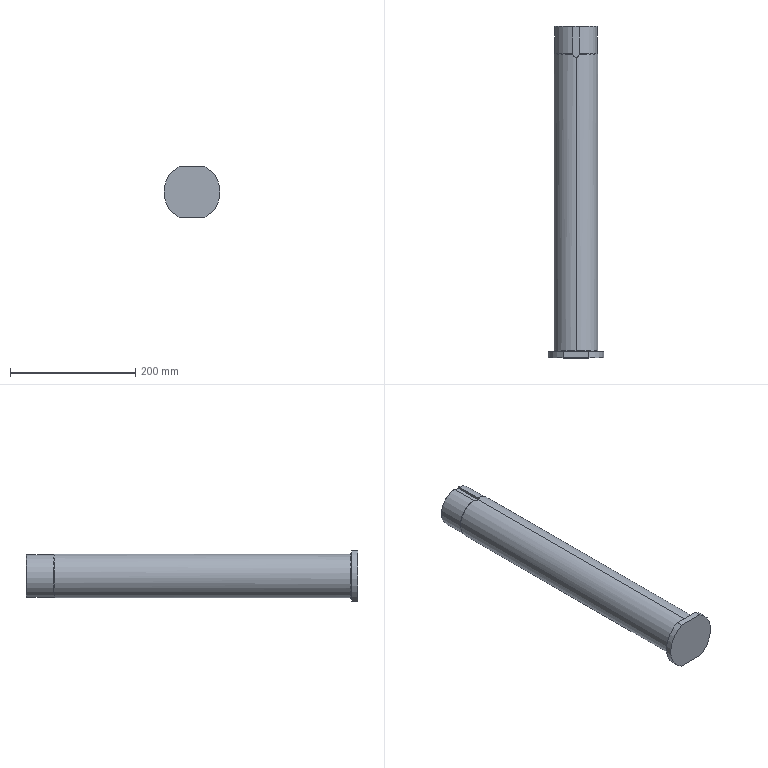Part | SolidWorks | features Fillet 2, ICE 2, Chamfer 1, Revolution 1 | 1 solid | 20 faces | box 90 x 530 x 80 mm | volume 2050473 mm3 | plane 8 | cylinder 6 | torus 4 | cone 2 | commonest cylinder face diameters 70 x2 90 x2 10 x1 68 x1
STEP:
#1=CARTESIAN_POINT('',(0.,10.,37.));
#2=VERTEX_POINT('',#1);
#3=CARTESIAN_POINT('',(0.,10.,-37.));
#4=VERTEX_POINT('',#3);
#5=CARTESIAN_POINT('',(0.,10.,0.));
#6=DIRECTION('',(0.,-1.,0.));
#7=DIRECTION('',(0.,0.,-1.));
#8=AXIS2_PLACEMENT_3D('',#5,#6,#7);
#9=CIRCLE('',#8,37.);
#10=EDGE_CURVE('',#2,#4,#9,.T.);
#11=ORIENTED_EDGE('',*,*,#10,.F.);
#12=CARTESIAN_POINT('',(0.,12.,35.));
#13=VERTEX_POINT('',#12);
#14=CARTESIAN_POINT('',(0.,12.,37.));
#15=DIRECTION('',(1.,0.,0.));
#16=DIRECTION('',(0.,0.,-1.));
#17=AXIS2_PLACEMENT_3D('',#14,#15,#16);
#18=CIRCLE('',#17,2.);
#19=EDGE_CURVE('',#2,#13,#18,.T.);
#20=ORIENTED_EDGE('',*,*,#19,.T.);
#21=CARTESIAN_POINT('',(0.,12.,-35.));
#22=VERTEX_POINT('',#21);
#23=CARTESIAN_POINT('',(0.,12.,0.));
#24=DIRECTION('',(0.,1.,0.));
#25=DIRECTION('',(0.,0.,-1.));
#26=AXIS2_PLACEMENT_3D('',#23,#24,#25);
#27=CIRCLE('',#26,35.);
#28=EDGE_CURVE('',#22,#13,#27,.T.);
#29=ORIENTED_EDGE('',*,*,#28,.F.);
#30=CARTESIAN_POINT('',(0.,12.,-37.));
#31=DIRECTION('',(-1.,0.,0.));
#32=DIRECTION('',(0.,0.,1.));
#33=AXIS2_PLACEMENT_3D('',#30,#31,#32);
#34=CIRCLE('',#33,2.);
#35=EDGE_CURVE('',#4,#22,#34,.T.);
#36=ORIENTED_EDGE('',*,*,#35,.F.);
#37=EDGE_LOOP('',(#11,#20,#29,#36));
#38=FACE_OUTER_BOUND('',#37,.T.);
#39=CARTESIAN_POINT('',(0.,12.,0.));
#40=DIRECTION('',(0.,-1.,0.));
#41=DIRECTION('',(0.,0.,-1.));
#42=AXIS2_PLACEMENT_3D('',#39,#40,#41);
#43=TOROIDAL_SURFACE('',#42,37.,2.);
#44=ADVANCED_FACE('',(#38),#43,.F.);
#45=CARTESIAN_POINT('',(5.,485.,34.641));
#46=VERTEX_POINT('',#45);
#47=CARTESIAN_POINT('',(0.,485.,-35.));
#48=VERTEX_POINT('',#47);
#49=CARTESIAN_POINT('',(0.,485.,0.));
#50=DIRECTION('',(0.,1.,0.));
#51=DIRECTION('',(0.,0.,1.));
#52=AXIS2_PLACEMENT_3D('',#49,#50,#51);
#53=CIRCLE('',#52,35.);
#54=EDGE_CURVE('',#46,#48,#53,.T.);
#55=ORIENTED_EDGE('',*,*,#54,.T.);
#56=CARTESIAN_POINT('',(0.,486.,-34.));
#57=VERTEX_POINT('',#56);
#58=CARTESIAN_POINT('',(0.,486.,-35.));
#59=DIRECTION('',(-1.,0.,0.));
#60=DIRECTION('',(0.,0.,1.));
#61=AXIS2_PLACEMENT_3D('',#58,#59,#60);
#62=CIRCLE('',#61,1.);
#63=EDGE_CURVE('',#48,#57,#62,.T.);
#64=ORIENTED_EDGE('',*,*,#63,.T.);
#65=CARTESIAN_POINT('',(5.,486.,33.63));
#66=VERTEX_POINT('',#65);
#67=CARTESIAN_POINT('',(0.,486.,0.));
#68=DIRECTION('',(0.,1.,0.));
#69=DIRECTION('',(0.,0.,-1.));
#70=AXIS2_PLACEMENT_3D('',#67,#68,#69);
#71=CIRCLE('',#70,34.);
#72=EDGE_CURVE('',#66,#57,#71,.T.);
#73=ORIENTED_EDGE('',*,*,#72,.F.);
#74=CARTESIAN_POINT('',(5.,485.,34.641));
#75=CARTESIAN_POINT('',(5.,485.,34.508));
#76=CARTESIAN_POINT('',(5.,485.026,34.378));
#77=CARTESIAN_POINT('',(5.,485.125,34.134));
#78=CARTESIAN_POINT('',(5.,485.199,34.022));
#79=CARTESIAN_POINT('',(5.,485.475,33.742));
#80=CARTESIAN_POINT('',(5.,485.734,33.63));
#81=CARTESIAN_POINT('',(5.,486.,33.63));
#82=B_SPLINE_CURVE_WITH_KNOTS('',3,(#74,#75,#76,#77,#78,#79,#80,#81),.UNSPECIFIED.,.F.,.F.,(4,2,2,4),(0.,0.0003926,0.0007852,0.00157),.UNSPECIFIED.);
#83=EDGE_CURVE('',#46,#66,#82,.T.);
#84=ORIENTED_EDGE('',*,*,#83,.F.);
#85=EDGE_LOOP('',(#55,#64,#73,#84));
#86=FACE_OUTER_BOUND('',#85,.T.);
#87=CARTESIAN_POINT('',(0.,486.,0.));
#88=DIRECTION('',(0.,-1.,0.));
#89=DIRECTION('',(0.,0.,-1.));
#90=AXIS2_PLACEMENT_3D('',#87,#88,#89);
#91=TOROIDAL_SURFACE('',#90,35.,1.);
#92=ADVANCED_FACE('',(#86),#91,.F.);
#93=CARTESIAN_POINT('',(0.,530.,-33.));
#94=VERTEX_POINT('',#93);
#95=CARTESIAN_POINT('',(-5.,530.,32.619));
#96=VERTEX_POINT('',#95);
#97=CARTESIAN_POINT('',(0.,530.,0.));
#98=DIRECTION('',(0.,1.,0.));
#99=DIRECTION('',(0.,0.,-1.));
#100=AXIS2_PLACEMENT_3D('',#97,#98,#99);
#101=CIRCLE('',#100,33.);
#102=EDGE_CURVE('',#94,#96,#101,.T.);
#103=ORIENTED_EDGE('',*,*,#102,.F.);
#104=CARTESIAN_POINT('',(0.,529.,-34.));
#105=VERTEX_POINT('',#104);
#106=CARTESIAN_POINT('',(0.,530.,-33.));
#107=DIRECTION('',(0.,-0.7071,-0.7071));
#108=VECTOR('',#107,1000.);
#109=LINE('',#106,#108);
#110=EDGE_CURVE('',#94,#105,#109,.T.);
#111=ORIENTED_EDGE('',*,*,#110,.T.);
#112=CARTESIAN_POINT('',(-5.,529.,33.63));
#113=VERTEX_POINT('',#112);
#114=CARTESIAN_POINT('',(0.,529.,0.));
#115=DIRECTION('',(0.,-1.,0.));
#116=DIRECTION('',(0.,0.,-1.));
#117=AXIS2_PLACEMENT_3D('',#114,#115,#116);
#118=CIRCLE('',#117,34.);
#119=EDGE_CURVE('',#113,#105,#118,.T.);
#120=ORIENTED_EDGE('',*,*,#119,.F.);
#121=CARTESIAN_POINT('',(-5.,530.,32.619));
#122=CARTESIAN_POINT('',(-5.,529.667,32.956));
#123=CARTESIAN_POINT('',(-5.,529.333,33.293));
#124=CARTESIAN_POINT('',(-5.,529.,33.63));
#125=B_SPLINE_CURVE_WITH_KNOTS('',3,(#121,#122,#123,#124),.UNSPECIFIED.,.F.,.F.,(4,4),(0.,0.001422),.UNSPECIFIED.);
#126=EDGE_CURVE('',#96,#113,#125,.T.);
#127=ORIENTED_EDGE('',*,*,#126,.F.);
#128=EDGE_LOOP('',(#103,#111,#120,#127));
#129=FACE_OUTER_BOUND('',#128,.T.);
#130=CARTESIAN_POINT('',(0.,530.,0.));
#131=DIRECTION('',(0.,-1.,0.));
#132=DIRECTION('',(0.,0.,-1.));
#133=AXIS2_PLACEMENT_3D('',#130,#131,#132);
#134=CONICAL_SURFACE('',#133,33.,0.7854);
#135=ADVANCED_FACE('',(#129),#134,.T.);
#136=CARTESIAN_POINT('',(0.,12.,0.));
#137=DIRECTION('',(0.,1.,0.));
#138=DIRECTION('',(0.,0.,-1.));
#139=AXIS2_PLACEMENT_3D('',#136,#137,#138);
#140=CIRCLE('',#139,35.);
#141=EDGE_CURVE('',#13,#22,#140,.T.);
#142=ORIENTED_EDGE('',*,*,#141,.T.);
#143=CARTESIAN_POINT('',(0.,0.,-35.));
#144=DIRECTION('',(0.,1.,0.));
#145=VECTOR('',#144,1000.);
#146=LINE('',#143,#145);
#147=EDGE_CURVE('',#22,#48,#146,.T.);
#148=ORIENTED_EDGE('',*,*,#147,.T.);
#149=ORIENTED_EDGE('',*,*,#54,.F.);
#150=CARTESIAN_POINT('',(0.,480.,35.));
#151=VERTEX_POINT('',#150);
#152=CARTESIAN_POINT('',(5.,485.,34.641));
#153=CARTESIAN_POINT('',(5.,484.669,34.641));
#154=CARTESIAN_POINT('',(4.967,484.344,34.646));
#155=CARTESIAN_POINT('',(4.872,483.864,34.659));
#156=CARTESIAN_POINT('',(4.832,483.705,34.665));
#157=CARTESIAN_POINT('',(4.737,483.391,34.678));
#158=CARTESIAN_POINT('',(4.681,483.235,34.686));
#159=CARTESIAN_POINT('',(4.492,482.781,34.711));
#160=CARTESIAN_POINT('',(4.339,482.494,34.731));
#161=CARTESIAN_POINT('',(3.976,481.95,34.774));
#162=CARTESIAN_POINT('',(3.765,481.693,34.798));
#163=CARTESIAN_POINT('',(3.304,481.233,34.845));
#164=CARTESIAN_POINT('',(3.052,481.026,34.868));
#165=CARTESIAN_POINT('',(2.505,480.66,34.911));
#166=CARTESIAN_POINT('',(2.215,480.505,34.931));
#167=CARTESIAN_POINT('',(1.613,480.256,34.964));
#168=CARTESIAN_POINT('',(1.297,480.16,34.977));
#169=CARTESIAN_POINT('',(0.6515,480.032,34.995));
#170=CARTESIAN_POINT('',(0.3267,480.,35.));
#171=CARTESIAN_POINT('',(0.,480.,35.));
#172=B_SPLINE_CURVE_WITH_KNOTS('',3,(#152,#153,#154,#155,#156,#157,#158,#159,#160,#161,#162,#163,#164,#165,#166,#167,#168,#169,#170,#171),.UNSPECIFIED.,.F.,.F.,(4,2,2,2,2,2,2,2,2,4),(0.,0.0009785,0.001468,0.001957,0.002935,0.003914,0.004892,0.005871,0.006849,0.007828),.UNSPECIFIED.);
#173=EDGE_CURVE('',#46,#151,#172,.T.);
#174=ORIENTED_EDGE('',*,*,#173,.T.);
#175=CARTESIAN_POINT('',(0.,0.,35.));
#176=DIRECTION('',(0.,1.,0.));
#177=VECTOR('',#176,1000.);
#178=LINE('',#175,#177);
#179=EDGE_CURVE('',#13,#151,#178,.T.);
#180=ORIENTED_EDGE('',*,*,#179,.F.);
#181=EDGE_LOOP('',(#142,#148,#149,#174,#180));
#182=FACE_OUTER_BOUND('',#181,.T.);
#183=CARTESIAN_POINT('',(0.,0.,0.));
#184=DIRECTION('',(0.,1.,0.));
#185=DIRECTION('',(0.,0.,1.));
#186=AXIS2_PLACEMENT_3D('',#183,#184,#185);
#187=CYLINDRICAL_SURFACE('',#186,35.);
#188=ADVANCED_FACE('',(#182),#187,.T.);
#189=ORIENTED_EDGE('',*,*,#147,.F.);
#190=ORIENTED_EDGE('',*,*,#28,.T.);
#191=ORIENTED_EDGE('',*,*,#179,.T.);
#192=CARTESIAN_POINT('',(-5.,485.,34.641));
#193=VERTEX_POINT('',#192);
#194=CARTESIAN_POINT('',(0.,480.,35.));
#195=CARTESIAN_POINT('',(-0.3264,480.,35.));
#196=CARTESIAN_POINT('',(-0.6579,480.033,34.995));
#197=CARTESIAN_POINT('',(-1.299,480.161,34.977));
#198=CARTESIAN_POINT('',(-1.611,480.255,34.964));
#199=CARTESIAN_POINT('',(-2.065,480.443,34.939));
#200=CARTESIAN_POINT('',(-2.215,480.514,34.93));
#201=CARTESIAN_POINT('',(-2.504,480.669,34.911));
#202=CARTESIAN_POINT('',(-2.643,480.753,34.9));
#203=CARTESIAN_POINT('',(-3.049,481.024,34.868));
#204=CARTESIAN_POINT('',(-3.302,481.231,34.845));
#205=CARTESIAN_POINT('',(-3.768,481.696,34.797));
#206=CARTESIAN_POINT('',(-3.974,481.948,34.774));
#207=CARTESIAN_POINT('',(-4.336,482.489,34.731));
#208=CARTESIAN_POINT('',(-4.493,482.781,34.711));
#209=CARTESIAN_POINT('',(-4.744,483.386,34.677));
#210=CARTESIAN_POINT('',(-4.838,483.697,34.664));
#211=CARTESIAN_POINT('',(-4.967,484.338,34.646));
#212=CARTESIAN_POINT('',(-5.,484.669,34.641));
#213=CARTESIAN_POINT('',(-5.,485.,34.641));
#214=B_SPLINE_CURVE_WITH_KNOTS('',3,(#194,#195,#196,#197,#198,#199,#200,#201,#202,#203,#204,#205,#206,#207,#208,#209,#210,#211,#212,#213),.UNSPECIFIED.,.F.,.F.,(4,2,2,2,2,2,2,2,2,4),(0.007828,0.008806,0.009783,0.01027,0.01076,0.01174,0.01272,0.01369,0.01467,0.01565),.UNSPECIFIED.);
#215=EDGE_CURVE('',#151,#193,#214,.T.);
#216=ORIENTED_EDGE('',*,*,#215,.T.);
#217=CARTESIAN_POINT('',(0.,485.,0.));
#218=DIRECTION('',(0.,1.,0.));
#219=DIRECTION('',(0.,0.,1.));
#220=AXIS2_PLACEMENT_3D('',#217,#218,#219);
#221=CIRCLE('',#220,35.);
#222=EDGE_CURVE('',#48,#193,#221,.T.);
#223=ORIENTED_EDGE('',*,*,#222,.F.);
#224=EDGE_LOOP('',(#189,#190,#191,#216,#223));
#225=FACE_OUTER_BOUND('',#224,.T.);
#226=CARTESIAN_POINT('',(0.,0.,0.));
#227=DIRECTION('',(0.,1.,0.));
#228=DIRECTION('',(0.,0.,1.));
#229=AXIS2_PLACEMENT_3D('',#226,#227,#228);
#230=CYLINDRICAL_SURFACE('',#229,35.);
#231=ADVANCED_FACE('',(#225),#230,.T.);
#232=CARTESIAN_POINT('',(5.,529.,33.63));
#233=VERTEX_POINT('',#232);
#234=CARTESIAN_POINT('',(5.,0.,33.63));
#235=DIRECTION('',(0.,-1.,0.));
#236=VECTOR('',#235,1000.);
#237=LINE('',#234,#236);
#238=EDGE_CURVE('',#233,#66,#237,.T.);
#239=ORIENTED_EDGE('',*,*,#238,.T.);
#240=ORIENTED_EDGE('',*,*,#72,.T.);
#241=CARTESIAN_POINT('',(-5.,486.,33.63));
#242=VERTEX_POINT('',#241);
#243=CARTESIAN_POINT('',(0.,486.,0.));
#244=DIRECTION('',(0.,1.,0.));
#245=DIRECTION('',(0.,0.,-1.));
#246=AXIS2_PLACEMENT_3D('',#243,#244,#245);
#247=CIRCLE('',#246,34.);
#248=EDGE_CURVE('',#57,#242,#247,.T.);
#249=ORIENTED_EDGE('',*,*,#248,.T.);
#250=CARTESIAN_POINT('',(-5.,0.,33.63));
#251=DIRECTION('',(0.,1.,0.));
#252=VECTOR('',#251,1000.);
#253=LINE('',#250,#252);
#254=EDGE_CURVE('',#242,#113,#253,.T.);
#255=ORIENTED_EDGE('',*,*,#254,.T.);
#256=ORIENTED_EDGE('',*,*,#119,.T.);
#257=CARTESIAN_POINT('',(0.,529.,0.));
#258=DIRECTION('',(0.,-1.,0.));
#259=DIRECTION('',(0.,0.,-1.));
#260=AXIS2_PLACEMENT_3D('',#257,#258,#259);
#261=CIRCLE('',#260,34.);
#262=EDGE_CURVE('',#105,#233,#261,.T.);
#263=ORIENTED_EDGE('',*,*,#262,.T.);
#264=EDGE_LOOP('',(#239,#240,#249,#255,#256,#263));
#265=FACE_OUTER_BOUND('',#264,.T.);
#266=CARTESIAN_POINT('',(0.,0.,0.));
#267=DIRECTION('',(0.,1.,0.));
#268=DIRECTION('',(0.,0.,1.));
#269=AXIS2_PLACEMENT_3D('',#266,#267,#268);
#270=CYLINDRICAL_SURFACE('',#269,34.);
#271=ADVANCED_FACE('',(#265),#270,.T.);
#272=CARTESIAN_POINT('',(5.,530.,30.));
#273=VERTEX_POINT('',#272);
#274=CARTESIAN_POINT('',(5.,530.,32.619));
#275=VERTEX_POINT('',#274);
#276=CARTESIAN_POINT('',(5.,530.,40.001));
#277=DIRECTION('',(0.,0.,1.));
#278=VECTOR('',#277,1000.);
#279=LINE('',#276,#278);
#280=EDGE_CURVE('',#273,#275,#279,.T.);
#281=ORIENTED_EDGE('',*,*,#280,.T.);
#282=CARTESIAN_POINT('',(0.,530.,0.));
#283=DIRECTION('',(0.,1.,0.));
#284=DIRECTION('',(0.,0.,-1.));
#285=AXIS2_PLACEMENT_3D('',#282,#283,#284);
#286=CIRCLE('',#285,33.);
#287=EDGE_CURVE('',#275,#94,#286,.T.);
#288=ORIENTED_EDGE('',*,*,#287,.T.);
#289=ORIENTED_EDGE('',*,*,#102,.T.);
#290=CARTESIAN_POINT('',(-5.,530.,30.));
#291=VERTEX_POINT('',#290);
#292=CARTESIAN_POINT('',(-5.,530.,40.001));
#293=DIRECTION('',(0.,0.,-1.));
#294=VECTOR('',#293,1000.);
#295=LINE('',#292,#294);
#296=EDGE_CURVE('',#96,#291,#295,.T.);
#297=ORIENTED_EDGE('',*,*,#296,.T.);
#298=CARTESIAN_POINT('',(0.,530.,30.));
#299=DIRECTION('',(1.,0.,0.));
#300=VECTOR('',#299,1000.);
#301=LINE('',#298,#300);
#302=EDGE_CURVE('',#291,#273,#301,.T.);
#303=ORIENTED_EDGE('',*,*,#302,.T.);
#304=EDGE_LOOP('',(#281,#288,#289,#297,#303));
#305=FACE_OUTER_BOUND('',#304,.T.);
#306=CARTESIAN_POINT('',(34.,530.,0.));
#307=DIRECTION('',(0.,-1.,0.));
#308=DIRECTION('',(0.,0.,-1.));
#309=AXIS2_PLACEMENT_3D('',#306,#307,#308);
#310=PLANE('',#309);
#311=ADVANCED_FACE('',(#305),#310,.F.);
#312=CARTESIAN_POINT('',(-20.616,0.,-40.));
#313=VERTEX_POINT('',#312);
#314=CARTESIAN_POINT('',(-20.616,0.,40.));
#315=VERTEX_POINT('',#314);
#316=CARTESIAN_POINT('',(0.,0.,0.));
#317=DIRECTION('',(0.,1.,0.));
#318=DIRECTION('',(0.,0.,1.));
#319=AXIS2_PLACEMENT_3D('',#316,#317,#318);
#320=CIRCLE('',#319,45.);
#321=EDGE_CURVE('',#313,#315,#320,.T.);
#322=ORIENTED_EDGE('',*,*,#321,.T.);
#323=CARTESIAN_POINT('',(-20.616,10.,40.));
#324=VERTEX_POINT('',#323);
#325=CARTESIAN_POINT('',(-20.616,0.,40.));
#326=DIRECTION('',(0.,1.,0.));
#327=VECTOR('',#326,1000.);
#328=LINE('',#325,#327);
#329=EDGE_CURVE('',#315,#324,#328,.T.);
#330=ORIENTED_EDGE('',*,*,#329,.T.);
#331=CARTESIAN_POINT('',(-20.616,10.,-40.));
#332=VERTEX_POINT('',#331);
#333=CARTESIAN_POINT('',(0.,10.,0.));
#334=DIRECTION('',(0.,1.,0.));
#335=DIRECTION('',(0.,0.,1.));
#336=AXIS2_PLACEMENT_3D('',#333,#334,#335);
#337=CIRCLE('',#336,45.);
#338=EDGE_CURVE('',#332,#324,#337,.T.);
#339=ORIENTED_EDGE('',*,*,#338,.F.);
#340=CARTESIAN_POINT('',(-20.616,0.,-40.));
#341=DIRECTION('',(0.,-1.,0.));
#342=VECTOR('',#341,1000.);
#343=LINE('',#340,#342);
#344=EDGE_CURVE('',#332,#313,#343,.T.);
#345=ORIENTED_EDGE('',*,*,#344,.T.);
#346=EDGE_LOOP('',(#322,#330,#339,#345));
#347=FACE_OUTER_BOUND('',#346,.T.);
#348=CARTESIAN_POINT('',(0.,0.,0.));
#349=DIRECTION('',(0.,1.,0.));
#350=DIRECTION('',(0.,0.,1.));
#351=AXIS2_PLACEMENT_3D('',#348,#349,#350);
#352=CYLINDRICAL_SURFACE('',#351,45.);
#353=ADVANCED_FACE('',(#347),#352,.T.);
#354=CARTESIAN_POINT('',(20.616,0.,40.));
#355=VERTEX_POINT('',#354);
#356=CARTESIAN_POINT('',(20.616,0.,-40.));
#357=VERTEX_POINT('',#356);
#358=CARTESIAN_POINT('',(0.,0.,0.));
#359=DIRECTION('',(0.,1.,0.));
#360=DIRECTION('',(0.,0.,1.));
#361=AXIS2_PLACEMENT_3D('',#358,#359,#360);
#362=CIRCLE('',#361,45.);
#363=EDGE_CURVE('',#355,#357,#362,.T.);
#364=ORIENTED_EDGE('',*,*,#363,.F.);
#365=CARTESIAN_POINT('',(65.,0.,40.));
#366=DIRECTION('',(1.,0.,0.));
#367=VECTOR('',#366,1000.);
#368=LINE('',#365,#367);
#369=EDGE_CURVE('',#315,#355,#368,.T.);
#370=ORIENTED_EDGE('',*,*,#369,.F.);
#371=ORIENTED_EDGE('',*,*,#321,.F.);
#372=CARTESIAN_POINT('',(65.,0.,-40.));
#373=DIRECTION('',(-1.,0.,0.));
#374=VECTOR('',#373,1000.);
#375=LINE('',#372,#374);
#376=EDGE_CURVE('',#357,#313,#375,.T.);
#377=ORIENTED_EDGE('',*,*,#376,.F.);
#378=EDGE_LOOP('',(#364,#370,#371,#377));
#379=FACE_OUTER_BOUND('',#378,.T.);
#380=CARTESIAN_POINT('',(0.,0.,0.));
#381=DIRECTION('',(0.,1.,0.));
#382=DIRECTION('',(0.,0.,1.));
#383=AXIS2_PLACEMENT_3D('',#380,#381,#382);
#384=PLANE('',#383);
#385=ADVANCED_FACE('',(#379),#384,.F.);
#386=CARTESIAN_POINT('',(20.616,10.,40.));
#387=VERTEX_POINT('',#386);
#388=CARTESIAN_POINT('',(20.616,10.,-40.));
#389=VERTEX_POINT('',#388);
#390=CARTESIAN_POINT('',(0.,10.,0.));
#391=DIRECTION('',(0.,1.,0.));
#392=DIRECTION('',(0.,0.,1.));
#393=AXIS2_PLACEMENT_3D('',#390,#391,#392);
#394=CIRCLE('',#393,45.);
#395=EDGE_CURVE('',#387,#389,#394,.T.);
#396=ORIENTED_EDGE('',*,*,#395,.F.);
#397=CARTESIAN_POINT('',(20.616,0.,40.));
#398=DIRECTION('',(0.,-1.,0.));
#399=VECTOR('',#398,1000.);
#400=LINE('',#397,#399);
#401=EDGE_CURVE('',#387,#355,#400,.T.);
#402=ORIENTED_EDGE('',*,*,#401,.T.);
#403=ORIENTED_EDGE('',*,*,#363,.T.);
#404=CARTESIAN_POINT('',(20.616,0.,-40.));
#405=DIRECTION('',(0.,1.,0.));
#406=VECTOR('',#405,1000.);
#407=LINE('',#404,#406);
#408=EDGE_CURVE('',#357,#389,#407,.T.);
#409=ORIENTED_EDGE('',*,*,#408,.T.);
#410=EDGE_LOOP('',(#396,#402,#403,#409));
#411=FACE_OUTER_BOUND('',#410,.T.);
#412=CARTESIAN_POINT('',(0.,0.,0.));
#413=DIRECTION('',(0.,1.,0.));
#414=DIRECTION('',(0.,0.,1.));
#415=AXIS2_PLACEMENT_3D('',#412,#413,#414);
#416=CYLINDRICAL_SURFACE('',#415,45.);
#417=ADVANCED_FACE('',(#411),#416,.T.);
#418=CARTESIAN_POINT('',(0.,10.,0.));
#419=DIRECTION('',(0.,-1.,0.));
#420=DIRECTION('',(0.,0.,-1.));
#421=AXIS2_PLACEMENT_3D('',#418,#419,#420);
#422=CIRCLE('',#421,37.);
#423=EDGE_CURVE('',#4,#2,#422,.T.);
#424=ORIENTED_EDGE('',*,*,#423,.T.);
#425=ORIENTED_EDGE('',*,*,#10,.T.);
#426=EDGE_LOOP('',(#424,#425));
#427=FACE_BOUND('',#426,.T.);
#428=ORIENTED_EDGE('',*,*,#338,.T.);
#429=CARTESIAN_POINT('',(45.,10.,40.));
#430=DIRECTION('',(1.,0.,0.));
#431=VECTOR('',#430,1000.);
#432=LINE('',#429,#431);
#433=EDGE_CURVE('',#324,#387,#432,.T.);
#434=ORIENTED_EDGE('',*,*,#433,.T.);
#435=ORIENTED_EDGE('',*,*,#395,.T.);
#436=CARTESIAN_POINT('',(45.,10.,-40.));
#437=DIRECTION('',(-1.,0.,0.));
#438=VECTOR('',#437,1000.);
#439=LINE('',#436,#438);
#440=EDGE_CURVE('',#389,#332,#439,.T.);
#441=ORIENTED_EDGE('',*,*,#440,.T.);
#442=EDGE_LOOP('',(#428,#434,#435,#441));
#443=FACE_OUTER_BOUND('',#442,.T.);
#444=CARTESIAN_POINT('',(45.,10.,0.));
#445=DIRECTION('',(0.,-1.,0.));
#446=DIRECTION('',(0.,0.,-1.));
#447=AXIS2_PLACEMENT_3D('',#444,#445,#446);
#448=PLANE('',#447);
#449=ADVANCED_FACE('',(#427,#443),#448,.F.);
#450=ORIENTED_EDGE('',*,*,#376,.T.);
#451=ORIENTED_EDGE('',*,*,#344,.F.);
#452=ORIENTED_EDGE('',*,*,#440,.F.);
#453=ORIENTED_EDGE('',*,*,#408,.F.);
#454=EDGE_LOOP('',(#450,#451,#452,#453));
#455=FACE_OUTER_BOUND('',#454,.T.);
#456=CARTESIAN_POINT('',(65.,10.,-40.));
#457=DIRECTION('',(0.,0.,1.));
#458=DIRECTION('',(1.,0.,0.));
#459=AXIS2_PLACEMENT_3D('',#456,#457,#458);
#460=PLANE('',#459);
#461=ADVANCED_FACE('',(#455),#460,.F.);
#462=ORIENTED_EDGE('',*,*,#369,.T.);
#463=ORIENTED_EDGE('',*,*,#401,.F.);
#464=ORIENTED_EDGE('',*,*,#433,.F.);
#465=ORIENTED_EDGE('',*,*,#329,.F.);
#466=EDGE_LOOP('',(#462,#463,#464,#465));
#467=FACE_OUTER_BOUND('',#466,.T.);
#468=CARTESIAN_POINT('',(65.,10.,40.));
#469=DIRECTION('',(0.,0.,-1.));
#470=DIRECTION('',(-1.,0.,0.));
#471=AXIS2_PLACEMENT_3D('',#468,#469,#470);
#472=PLANE('',#471);
#473=ADVANCED_FACE('',(#467),#472,.F.);
#474=ORIENTED_EDGE('',*,*,#296,.F.);
#475=ORIENTED_EDGE('',*,*,#126,.T.);
#476=ORIENTED_EDGE('',*,*,#254,.F.);
#477=CARTESIAN_POINT('',(-5.,486.,33.63));
#478=CARTESIAN_POINT('',(-5.,485.867,33.63));
#479=CARTESIAN_POINT('',(-5.,485.737,33.657));
#480=CARTESIAN_POINT('',(-5.,485.494,33.759));
#481=CARTESIAN_POINT('',(-5.,485.383,33.835));
#482=CARTESIAN_POINT('',(-5.,485.199,34.021));
#483=CARTESIAN_POINT('',(-5.,485.125,34.134));
#484=CARTESIAN_POINT('',(-5.,485.026,34.376));
#485=CARTESIAN_POINT('',(-5.,485.,34.508));
#486=CARTESIAN_POINT('',(-5.,485.,34.641));
#487=B_SPLINE_CURVE_WITH_KNOTS('',3,(#477,#478,#479,#480,#481,#482,#483,#484,#485,#486),.UNSPECIFIED.,.F.,.F.,(4,2,2,2,4),(0.,0.0003926,0.0007852,0.001178,0.00157),.UNSPECIFIED.);
#488=EDGE_CURVE('',#242,#193,#487,.T.);
#489=ORIENTED_EDGE('',*,*,#488,.T.);
#490=CARTESIAN_POINT('',(-5.,485.,30.));
#491=VERTEX_POINT('',#490);
#492=CARTESIAN_POINT('',(-5.,485.,40.001));
#493=DIRECTION('',(0.,0.,-1.));
#494=VECTOR('',#493,1000.);
#495=LINE('',#492,#494);
#496=EDGE_CURVE('',#193,#491,#495,.T.);
#497=ORIENTED_EDGE('',*,*,#496,.T.);
#498=CARTESIAN_POINT('',(-5.,530.,30.));
#499=DIRECTION('',(0.,-1.,0.));
#500=VECTOR('',#499,1000.);
#501=LINE('',#498,#500);
#502=EDGE_CURVE('',#291,#491,#501,.T.);
#503=ORIENTED_EDGE('',*,*,#502,.F.);
#504=EDGE_LOOP('',(#474,#475,#476,#489,#497,#503));
#505=FACE_OUTER_BOUND('',#504,.T.);
#506=CARTESIAN_POINT('',(-5.,530.,40.001));
#507=DIRECTION('',(1.,0.,0.));
#508=DIRECTION('',(0.,1.,0.));
#509=AXIS2_PLACEMENT_3D('',#506,#507,#508);
#510=PLANE('',#509);
#511=ADVANCED_FACE('',(#505),#510,.T.);
#512=ORIENTED_EDGE('',*,*,#173,.F.);
#513=CARTESIAN_POINT('',(5.,485.,30.));
#514=VERTEX_POINT('',#513);
#515=CARTESIAN_POINT('',(5.,485.,40.001));
#516=DIRECTION('',(0.,0.,-1.));
#517=VECTOR('',#516,1000.);
#518=LINE('',#515,#517);
#519=EDGE_CURVE('',#46,#514,#518,.T.);
#520=ORIENTED_EDGE('',*,*,#519,.T.);
#521=CARTESIAN_POINT('',(0.,485.,30.));
#522=DIRECTION('',(0.,0.,1.));
#523=DIRECTION('',(1.,0.,0.));
#524=AXIS2_PLACEMENT_3D('',#521,#522,#523);
#525=CIRCLE('',#524,5.);
#526=EDGE_CURVE('',#491,#514,#525,.T.);
#527=ORIENTED_EDGE('',*,*,#526,.F.);
#528=ORIENTED_EDGE('',*,*,#496,.F.);
#529=ORIENTED_EDGE('',*,*,#215,.F.);
#530=EDGE_LOOP('',(#512,#520,#527,#528,#529));
#531=FACE_OUTER_BOUND('',#530,.T.);
#532=CARTESIAN_POINT('',(0.,485.,40.001));
#533=DIRECTION('',(0.,0.,-1.));
#534=DIRECTION('',(-1.,0.,0.));
#535=AXIS2_PLACEMENT_3D('',#532,#533,#534);
#536=CYLINDRICAL_SURFACE('',#535,5.);
#537=ADVANCED_FACE('',(#531),#536,.F.);
#538=ORIENTED_EDGE('',*,*,#238,.F.);
#539=CARTESIAN_POINT('',(5.,529.,33.63));
#540=CARTESIAN_POINT('',(5.,529.333,33.293));
#541=CARTESIAN_POINT('',(5.,529.667,32.956));
#542=CARTESIAN_POINT('',(5.,530.,32.619));
#543=B_SPLINE_CURVE_WITH_KNOTS('',3,(#539,#540,#541,#542),.UNSPECIFIED.,.F.,.F.,(4,4),(0.,0.001422),.UNSPECIFIED.);
#544=EDGE_CURVE('',#233,#275,#543,.T.);
#545=ORIENTED_EDGE('',*,*,#544,.T.);
#546=ORIENTED_EDGE('',*,*,#280,.F.);
#547=CARTESIAN_POINT('',(5.,530.,30.));
#548=DIRECTION('',(0.,1.,0.));
#549=VECTOR('',#548,1000.);
#550=LINE('',#547,#549);
#551=EDGE_CURVE('',#514,#273,#550,.T.);
#552=ORIENTED_EDGE('',*,*,#551,.F.);
#553=ORIENTED_EDGE('',*,*,#519,.F.);
#554=ORIENTED_EDGE('',*,*,#83,.T.);
#555=EDGE_LOOP('',(#538,#545,#546,#552,#553,#554));
#556=FACE_OUTER_BOUND('',#555,.T.);
#557=CARTESIAN_POINT('',(5.,530.,40.001));
#558=DIRECTION('',(-1.,0.,0.));
#559=DIRECTION('',(0.,-1.,0.));
#560=AXIS2_PLACEMENT_3D('',#557,#558,#559);
#561=PLANE('',#560);
#562=ADVANCED_FACE('',(#556),#561,.T.);
#563=ORIENTED_EDGE('',*,*,#502,.T.);
#564=ORIENTED_EDGE('',*,*,#526,.T.);
#565=ORIENTED_EDGE('',*,*,#551,.T.);
#566=ORIENTED_EDGE('',*,*,#302,.F.);
#567=EDGE_LOOP('',(#563,#564,#565,#566));
#568=FACE_OUTER_BOUND('',#567,.T.);
#569=CARTESIAN_POINT('',(0.,530.,30.));
#570=DIRECTION('',(0.,0.,1.));
#571=DIRECTION('',(1.,0.,0.));
#572=AXIS2_PLACEMENT_3D('',#569,#570,#571);
#573=PLANE('',#572);
#574=ADVANCED_FACE('',(#568),#573,.T.);
#575=ORIENTED_EDGE('',*,*,#110,.F.);
#576=ORIENTED_EDGE('',*,*,#287,.F.);
#577=ORIENTED_EDGE('',*,*,#544,.F.);
#578=ORIENTED_EDGE('',*,*,#262,.F.);
#579=EDGE_LOOP('',(#575,#576,#577,#578));
#580=FACE_OUTER_BOUND('',#579,.T.);
#581=CARTESIAN_POINT('',(0.,530.,0.));
#582=DIRECTION('',(0.,-1.,0.));
#583=DIRECTION('',(0.,0.,-1.));
#584=AXIS2_PLACEMENT_3D('',#581,#582,#583);
#585=CONICAL_SURFACE('',#584,33.,0.7854);
#586=ADVANCED_FACE('',(#580),#585,.T.);
#587=ORIENTED_EDGE('',*,*,#63,.F.);
#588=ORIENTED_EDGE('',*,*,#222,.T.);
#589=ORIENTED_EDGE('',*,*,#488,.F.);
#590=ORIENTED_EDGE('',*,*,#248,.F.);
#591=EDGE_LOOP('',(#587,#588,#589,#590));
#592=FACE_OUTER_BOUND('',#591,.T.);
#593=CARTESIAN_POINT('',(0.,486.,0.));
#594=DIRECTION('',(0.,-1.,0.));
#595=DIRECTION('',(0.,0.,-1.));
#596=AXIS2_PLACEMENT_3D('',#593,#594,#595);
#597=TOROIDAL_SURFACE('',#596,35.,1.);
#598=ADVANCED_FACE('',(#592),#597,.F.);
#599=ORIENTED_EDGE('',*,*,#19,.F.);
#600=ORIENTED_EDGE('',*,*,#423,.F.);
#601=ORIENTED_EDGE('',*,*,#35,.T.);
#602=ORIENTED_EDGE('',*,*,#141,.F.);
#603=EDGE_LOOP('',(#599,#600,#601,#602));
#604=FACE_OUTER_BOUND('',#603,.T.);
#605=CARTESIAN_POINT('',(0.,12.,0.));
#606=DIRECTION('',(0.,-1.,0.));
#607=DIRECTION('',(0.,0.,-1.));
#608=AXIS2_PLACEMENT_3D('',#605,#606,#607);
#609=TOROIDAL_SURFACE('',#608,37.,2.);
#610=ADVANCED_FACE('',(#604),#609,.F.);
#611=CLOSED_SHELL('',(#44,#92,#135,#188,#231,#271,#311,#353,#385,#417,#449,#461,#473,#511,#537,#562,#574,#586,#598,#610));
#612=MANIFOLD_SOLID_BREP('',#611);
#613=CARTESIAN_POINT('',(0.,0.,0.));
#614=DIRECTION('',(0.,0.,1.));
#615=DIRECTION('',(1.,0.,0.));
#616=AXIS2_PLACEMENT_3D('',#613,#614,#615);
#617=(LENGTH_UNIT()NAMED_UNIT(*)SI_UNIT(.MILLI.,.METRE.));
#618=UNCERTAINTY_MEASURE_WITH_UNIT(LENGTH_MEASURE(0.00001),#617,'','');
#619=(NAMED_UNIT(*)PLANE_ANGLE_UNIT()SI_UNIT($,.RADIAN.));
#620=(NAMED_UNIT(*)SI_UNIT($,.STERADIAN.)SOLID_ANGLE_UNIT());
#621=(GEOMETRIC_REPRESENTATION_CONTEXT(3)GLOBAL_UNCERTAINTY_ASSIGNED_CONTEXT((#618))GLOBAL_UNIT_ASSIGNED_CONTEXT((#617,#619,#620))REPRESENTATION_CONTEXT('',''));
#622=ADVANCED_BREP_SHAPE_REPRESENTATION('',(#612,#616),#621);